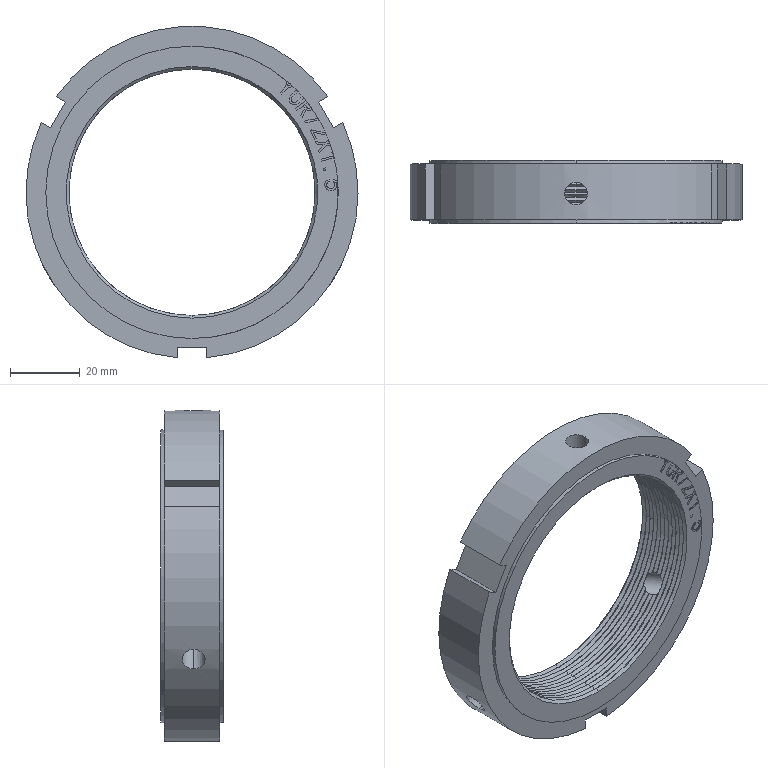Part | STEP file | YCR72x1.5 Radial Lock Nut | 1 solid | 168 faces | box 95 x 18 x 94.809 mm | volume 50193 mm3 | plane 74 | cone 62 | spline 21 | cylinder 11 | commonest cylinder face diameters 6.5 x6 95 x3 83.65 x2